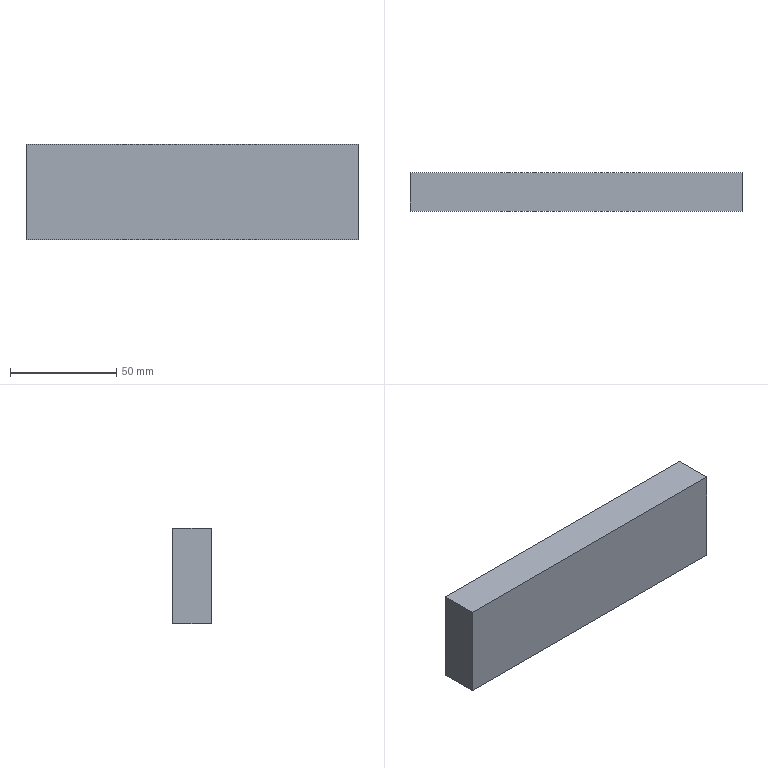NC program | NX | posted with a generic post | part box 156 x 18 x 45 mm
Lines 1295 to 2242 of 3545:
(PLANAR_PROFILING , TOOL : D8C)
N2540 T06 M6
N2542 G53
N2544 G17 G0 G90 X-157.794 Y11.317 S3500 M3
N2546 G43 Z19.87 H6
N2548 Z2.8
N2550 G94 G1 Z-0.2 F2000.
N2552 G3 X-152.934 Y11.934 R4.
N2554 G1 X-151.934 Y12.934
N2556 G2 X-149. Y14.15 R4.15
N2558 G1 X-27.15
N2560 Y39.
N2562 G2 X-25.934 Y41.934 R4.15
N2564 G1 X-24.934 Y42.934
N2566 G2 X-22. Y44.15 R4.15
N2568 G1 X-1.
N2570 G2 X1.934 Y42.934 R4.15
N2572 G1 X2.934 Y41.934
N2574 G3 X7.794 Y41.317 R4.
N2576 G1 Z2.8
N2578 G0 Z2.6
N2580 G1 Z-0.4
N2582 G2 X2.934 Y41.934 R4.
N2584 G1 X1.934 Y42.934
N2586 G3 X-1. Y44.15 R4.15
N2588 G1 X-22.
N2590 G3 X-24.934 Y42.934 R4.15
N2592 G1 X-25.934 Y41.934
N2594 G3 X-27.15 Y39. R4.15
N2596 G1 Y14.15
N2598 X-149.
N2600 G3 X-151.934 Y12.934 R4.15
N2602 G1 X-152.934 Y11.934
N2604 G2 X-157.794 Y11.317 R4.
N2606 G1 Z2.6
N2608 G0 Z2.4
N2610 G1 Z-0.6
N2612 G3 X-152.934 Y11.934 R4.
N2614 G1 X-151.934 Y12.934
N2616 G2 X-149. Y14.15 R4.15
N2618 G1 X-27.15
N2620 Y39.
N2622 G2 X-25.934 Y41.934 R4.15
N2624 G1 X-24.934 Y42.934
N2626 G2 X-22. Y44.15 R4.15
N2628 G1 X-1.
N2630 G2 X1.934 Y42.934 R4.15
N2632 G1 X2.934 Y41.934
N2634 G3 X7.794 Y41.317 R4.
N2636 G1 Z2.4
N2638 G0 Z2.2
N2640 G1 Z-0.8
N2642 G2 X2.934 Y41.934 R4.
N2644 G1 X1.934 Y42.934
N2646 G3 X-1. Y44.15 R4.15
N2648 G1 X-22.
N2650 G3 X-24.934 Y42.934 R4.15
N2652 G1 X-25.934 Y41.934
N2654 G3 X-27.15 Y39. R4.15
N2656 G1 Y14.15
N2658 X-149.
N2660 G3 X-151.934 Y12.934 R4.15
N2662 G1 X-152.934 Y11.934
N2664 G2 X-157.794 Y11.317 R4.
N2666 G1 Z2.2
N2668 G0 Z2.
N2670 G1 Z-1.
N2672 G3 X-152.934 Y11.934 R4.
N2674 G1 X-151.934 Y12.934
N2676 G2 X-149. Y14.15 R4.15
N2678 G1 X-27.15
N2680 Y39.
N2682 G2 X-25.934 Y41.934 R4.15
N2684 G1 X-24.934 Y42.934
N2686 G2 X-22. Y44.15 R4.15
N2688 G1 X-1.
N2690 G2 X1.934 Y42.934 R4.15
N2692 G1 X2.934 Y41.934
N2694 G3 X7.794 Y41.317 R4.
N2696 G1 Z2.
N2698 G0 Z1.8
N2700 G1 Z-1.2
N2702 G2 X2.934 Y41.934 R4.
N2704 G1 X1.934 Y42.934
N2706 G3 X-1. Y44.15 R4.15
N2708 G1 X-22.
N2710 G3 X-24.934 Y42.934 R4.15
N2712 G1 X-25.934 Y41.934
N2714 G3 X-27.15 Y39. R4.15
N2716 G1 Y14.15
N2718 X-149.
N2720 G3 X-151.934 Y12.934 R4.15
N2722 G1 X-152.934 Y11.934
N2724 G2 X-157.794 Y11.317 R4.
N2726 G1 Z1.8
N2728 G0 Z1.6
N2730 G1 Z-1.4
N2732 G3 X-152.934 Y11.934 R4.
N2734 G1 X-151.934 Y12.934
N2736 G2 X-149. Y14.15 R4.15
N2738 G1 X-27.15
N2740 Y39.
N2742 G2 X-25.934 Y41.934 R4.15
N2744 G1 X-24.934 Y42.934
N2746 G2 X-22. Y44.15 R4.15
N2748 G1 X-1.
N2750 G2 X1.934 Y42.934 R4.15
N2752 G1 X2.934 Y41.934
N2754 G3 X7.794 Y41.317 R4.
N2756 G1 Z1.6
N2758 G0 Z1.4
N2760 G1 Z-1.6
N2762 G2 X2.934 Y41.934 R4.
N2764 G1 X1.934 Y42.934
N2766 G3 X-1. Y44.15 R4.15
N2768 G1 X-22.
N2770 G3 X-24.934 Y42.934 R4.15
N2772 G1 X-25.934 Y41.934
N2774 G3 X-27.15 Y39. R4.15
N2776 G1 Y14.15
N2778 X-149.
N2780 G3 X-151.934 Y12.934 R4.15
N2782 G1 X-152.934 Y11.934
N2784 G2 X-157.794 Y11.317 R4.
N2786 G1 Z1.4
N2788 G0 Z1.2
N2790 G1 Z-1.8
N2792 G3 X-152.934 Y11.934 R4.
N2794 G1 X-151.934 Y12.934
N2796 G2 X-149. Y14.15 R4.15
N2798 G1 X-27.15
N2800 Y39.
N2802 G2 X-25.934 Y41.934 R4.15
N2804 G1 X-24.934 Y42.934
N2806 G2 X-22. Y44.15 R4.15
N2808 G1 X-1.
N2810 G2 X1.934 Y42.934 R4.15
N2812 G1 X2.934 Y41.934
N2814 G3 X7.794 Y41.317 R4.
N2816 G1 Z1.2
N2818 G0 Z1.
N2820 G1 Z-2.
N2822 G2 X2.934 Y41.934 R4.
N2824 G1 X1.934 Y42.934
N2826 G3 X-1. Y44.15 R4.15
N2828 G1 X-22.
N2830 G3 X-24.934 Y42.934 R4.15
N2832 G1 X-25.934 Y41.934
N2834 G3 X-27.15 Y39. R4.15
N2836 G1 Y14.15
N2838 X-149.
N2840 G3 X-151.934 Y12.934 R4.15
N2842 G1 X-152.934 Y11.934
N2844 G2 X-157.794 Y11.317 R4.
N2846 G1 Z1.
N2848 G0 Z0.8
N2850 G1 Z-2.2
N2852 G3 X-152.934 Y11.934 R4.
N2854 G1 X-151.934 Y12.934
N2856 G2 X-149. Y14.15 R4.15
N2858 G1 X-27.15
N2860 Y39.
N2862 G2 X-25.934 Y41.934 R4.15
N2864 G1 X-24.934 Y42.934
N2866 G2 X-22. Y44.15 R4.15
N2868 G1 X-1.
N2870 G2 X1.934 Y42.934 R4.15
N2872 G1 X2.934 Y41.934
N2874 G3 X7.794 Y41.317 R4.
N2876 G1 Z0.8
N2878 G0 Z0.6
N2880 G1 Z-2.4
N2882 G2 X2.934 Y41.934 R4.
N2884 G1 X1.934 Y42.934
N2886 G3 X-1. Y44.15 R4.15
N2888 G1 X-22.
N2890 G3 X-24.934 Y42.934 R4.15
N2892 G1 X-25.934 Y41.934
N2894 G3 X-27.15 Y39. R4.15
N2896 G1 Y14.15
N2898 X-149.
N2900 G3 X-151.934 Y12.934 R4.15
N2902 G1 X-152.934 Y11.934
N2904 G2 X-157.794 Y11.317 R4.
N2906 G1 Z0.6
N2908 G0 Z0.4
N2910 G1 Z-2.6
N2912 G3 X-152.934 Y11.934 R4.
N2914 G1 X-151.934 Y12.934
N2916 G2 X-149. Y14.15 R4.15
N2918 G1 X-27.15
N2920 Y39.
N2922 G2 X-25.934 Y41.934 R4.15
N2924 G1 X-24.934 Y42.934
N2926 G2 X-22. Y44.15 R4.15
N2928 G1 X-1.
N2930 G2 X1.934 Y42.934 R4.15
N2932 G1 X2.934 Y41.934
N2934 G3 X7.794 Y41.317 R4.
N2936 G1 Z0.4
N2938 G0 Z0.2
N2940 G1 Z-2.8
N2942 G2 X2.934 Y41.934 R4.
N2944 G1 X1.934 Y42.934
N2946 G3 X-1. Y44.15 R4.15
N2948 G1 X-22.
N2950 G3 X-24.934 Y42.934 R4.15
N2952 G1 X-25.934 Y41.934
N2954 G3 X-27.15 Y39. R4.15
N2956 G1 Y14.15
N2958 X-149.
N2960 G3 X-151.934 Y12.934 R4.15
N2962 G1 X-152.934 Y11.934
N2964 G2 X-157.794 Y11.317 R4.
N2966 G1 Z0.2
N2968 G0 Z0.
N2970 G1 Z-3.
N2972 G3 X-152.934 Y11.934 R4.
N2974 G1 X-151.934 Y12.934
N2976 G2 X-149. Y14.15 R4.15
N2978 G1 X-27.15
N2980 Y39.
N2982 G2 X-25.934 Y41.934 R4.15
N2984 G1 X-24.934 Y42.934
N2986 G2 X-22. Y44.15 R4.15
N2988 G1 X-1.
N2990 G2 X1.934 Y42.934 R4.15
N2992 G1 X2.934 Y41.934
N2994 G3 X7.794 Y41.317 R4.
N2996 G1 Z0.
N2998 G0 Z-0.2
N3000 G1 Z-3.2
N3002 G2 X2.934 Y41.934 R4.
N3004 G1 X1.934 Y42.934
N3006 G3 X-1. Y44.15 R4.15
N3008 G1 X-22.
N3010 G3 X-24.934 Y42.934 R4.15
N3012 G1 X-25.934 Y41.934
N3014 G3 X-27.15 Y39. R4.15
N3016 G1 Y14.15
N3018 X-149.
N3020 G3 X-151.934 Y12.934 R4.15
N3022 G1 X-152.934 Y11.934
N3024 G2 X-157.794 Y11.317 R4.
N3026 G1 Z-0.2
N3028 G0 Z-0.4
N3030 G1 Z-3.4
N3032 G3 X-152.934 Y11.934 R4.
N3034 G1 X-151.934 Y12.934
N3036 G2 X-149. Y14.15 R4.15
N3038 G1 X-27.15
N3040 Y39.
N3042 G2 X-25.934 Y41.934 R4.15
N3044 G1 X-24.934 Y42.934
N3046 G2 X-22. Y44.15 R4.15
N3048 G1 X-1.
N3050 G2 X1.934 Y42.934 R4.15
N3052 G1 X2.934 Y41.934
N3054 G3 X7.794 Y41.317 R4.
N3056 G1 Z-0.4
N3058 G0 Z-0.6
N3060 G1 Z-3.6
N3062 G2 X2.934 Y41.934 R4.
N3064 G1 X1.934 Y42.934
N3066 G3 X-1. Y44.15 R4.15
N3068 G1 X-22.
N3070 G3 X-24.934 Y42.934 R4.15
N3072 G1 X-25.934 Y41.934
N3074 G3 X-27.15 Y39. R4.15
N3076 G1 Y14.15
N3078 X-149.
N3080 G3 X-151.934 Y12.934 R4.15
N3082 G1 X-152.934 Y11.934
N3084 G2 X-157.794 Y11.317 R4.
N3086 G1 Z-0.6
N3088 G0 Z-0.8
N3090 G1 Z-3.8
N3092 G3 X-152.934 Y11.934 R4.
N3094 G1 X-151.934 Y12.934
N3096 G2 X-149. Y14.15 R4.15
N3098 G1 X-27.15
N3100 Y39.
N3102 G2 X-25.934 Y41.934 R4.15
N3104 G1 X-24.934 Y42.934
N3106 G2 X-22. Y44.15 R4.15
N3108 G1 X-1.
N3110 G2 X1.934 Y42.934 R4.15
N3112 G1 X2.934 Y41.934
N3114 G3 X7.794 Y41.317 R4.
N3116 G1 Z-0.8
N3118 G0 Z-1.
N3120 G1 Z-4.
N3122 G2 X2.934 Y41.934 R4.
N3124 G1 X1.934 Y42.934
N3126 G3 X-1. Y44.15 R4.15
N3128 G1 X-22.
N3130 G3 X-24.934 Y42.934 R4.15
N3132 G1 X-25.934 Y41.934
N3134 G3 X-27.15 Y39. R4.15
N3136 G1 Y14.15
N3138 X-149.
N3140 G3 X-151.934 Y12.934 R4.15
N3142 G1 X-152.934 Y11.934
N3144 G2 X-157.794 Y11.317 R4.
N3146 G1 Z-1.
N3148 G0 Z-1.2
N3150 G1 Z-4.2
N3152 G3 X-152.934 Y11.934 R4.
N3154 G1 X-151.934 Y12.934
N3156 G2 X-149. Y14.15 R4.15
N3158 G1 X-27.15
N3160 Y39.
N3162 G2 X-25.934 Y41.934 R4.15
N3164 G1 X-24.934 Y42.934
N3166 G2 X-22. Y44.15 R4.15
N3168 G1 X-1.
N3170 G2 X1.934 Y42.934 R4.15
N3172 G1 X2.934 Y41.934
N3174 G3 X7.794 Y41.317 R4.
N3176 G1 Z-1.2
N3178 G0 Z-1.4
N3180 G1 Z-4.4
N3182 G2 X2.934 Y41.934 R4.
N3184 G1 X1.934 Y42.934
N3186 G3 X-1. Y44.15 R4.15
N3188 G1 X-22.
N3190 G3 X-24.934 Y42.934 R4.15
N3192 G1 X-25.934 Y41.934
N3194 G3 X-27.15 Y39. R4.15
N3196 G1 Y14.15
N3198 X-149.
N3200 G3 X-151.934 Y12.934 R4.15
N3202 G1 X-152.934 Y11.934
N3204 G2 X-157.794 Y11.317 R4.
N3206 G1 Z-1.4
N3208 G0 Z-1.6
N3210 G1 Z-4.6
N3212 G3 X-152.934 Y11.934 R4.
N3214 G1 X-151.934 Y12.934
N3216 G2 X-149. Y14.15 R4.15
N3218 G1 X-27.15
N3220 Y39.
N3222 G2 X-25.934 Y41.934 R4.15
N3224 G1 X-24.934 Y42.934
N3226 G2 X-22. Y44.15 R4.15
N3228 G1 X-1.
N3230 G2 X1.934 Y42.934 R4.15
N3232 G1 X2.934 Y41.934
N3234 G3 X7.794 Y41.317 R4.
N3236 G1 Z-1.6
N3238 G0 Z-1.8
N3240 G1 Z-4.8
N3242 G2 X2.934 Y41.934 R4.
N3244 G1 X1.934 Y42.934
N3246 G3 X-1. Y44.15 R4.15
N3248 G1 X-22.
N3250 G3 X-24.934 Y42.934 R4.15
N3252 G1 X-25.934 Y41.934
N3254 G3 X-27.15 Y39. R4.15
N3256 G1 Y14.15
N3258 X-149.
N3260 G3 X-151.934 Y12.934 R4.15
N3262 G1 X-152.934 Y11.934
N3264 G2 X-157.794 Y11.317 R4.
N3266 G1 Z-1.8
N3268 G0 Z-2.
N3270 G1 Z-5.
N3272 G3 X-152.934 Y11.934 R4.
N3274 G1 X-151.934 Y12.934
N3276 G2 X-149. Y14.15 R4.15
N3278 G1 X-27.15
N3280 Y39.
N3282 G2 X-25.934 Y41.934 R4.15
N3284 G1 X-24.934 Y42.934
N3286 G2 X-22. Y44.15 R4.15
N3288 G1 X-1.
N3290 G2 X1.934 Y42.934 R4.15
N3292 G1 X2.934 Y41.934
N3294 G3 X7.794 Y41.317 R4.
N3296 G1 Z-2.
N3298 G0 Z-2.2
N3300 G1 Z-5.2
N3302 G2 X2.934 Y41.934 R4.
N3304 G1 X1.934 Y42.934
N3306 G3 X-1. Y44.15 R4.15
N3308 G1 X-22.
N3310 G3 X-24.934 Y42.934 R4.15
N3312 G1 X-25.934 Y41.934
N3314 G3 X-27.15 Y39. R4.15
N3316 G1 Y14.15
N3318 X-149.
N3320 G3 X-151.934 Y12.934 R4.15
N3322 G1 X-152.934 Y11.934
N3324 G2 X-157.794 Y11.317 R4.
N3326 G1 Z-2.2
N3328 G0 Z-2.4
N3330 G1 Z-5.4
N3332 G3 X-152.934 Y11.934 R4.
N3334 G1 X-151.934 Y12.934
N3336 G2 X-149. Y14.15 R4.15
N3338 G1 X-27.15
N3340 Y39.
N3342 G2 X-25.934 Y41.934 R4.15
N3344 G1 X-24.934 Y42.934
N3346 G2 X-22. Y44.15 R4.15
N3348 G1 X-1.
N3350 G2 X1.934 Y42.934 R4.15
N3352 G1 X2.934 Y41.934
N3354 G3 X7.794 Y41.317 R4.
N3356 G1 Z-2.4
N3358 G0 Z-2.6
N3360 G1 Z-5.6
N3362 G2 X2.934 Y41.934 R4.
N3364 G1 X1.934 Y42.934
N3366 G3 X-1. Y44.15 R4.15
N3368 G1 X-22.
N3370 G3 X-24.934 Y42.934 R4.15
N3372 G1 X-25.934 Y41.934
N3374 G3 X-27.15 Y39. R4.15
N3376 G1 Y14.15
N3378 X-149.
N3380 G3 X-151.934 Y12.934 R4.15
N3382 G1 X-152.934 Y11.934
N3384 G2 X-157.794 Y11.317 R4.
N3386 G1 Z-2.6
N3388 G0 Z-2.8
N3390 G1 Z-5.8
N3392 G3 X-152.934 Y11.934 R4.
N3394 G1 X-151.934 Y12.934
N3396 G2 X-149. Y14.15 R4.15
N3398 G1 X-27.15
N3400 Y39.
N3402 G2 X-25.934 Y41.934 R4.15
N3404 G1 X-24.934 Y42.934
N3406 G2 X-22. Y44.15 R4.15
N3408 G1 X-1.
N3410 G2 X1.934 Y42.934 R4.15
N3412 G1 X2.934 Y41.934
N3414 G3 X7.794 Y41.317 R4.
N3416 G1 Z-2.8
N3418 G0 Z-3.
N3420 G1 Z-6.
N3422 G2 X2.934 Y41.934 R4.
N3424 G1 X1.934 Y42.934
N3426 G3 X-1. Y44.15 R4.15
N3428 G1 X-22.
N3430 G3 X-24.934 Y42.934 R4.15
N3432 G1 X-25.934 Y41.934
N3434 G3 X-27.15 Y39. R4.15
N3436 G1 Y14.15
N3438 X-149.
N3440 G3 X-151.934 Y12.934 R4.15
N3442 G1 X-152.934 Y11.934
N3444 G2 X-157.794 Y11.317 R4.
N3446 G1 Z-3.
N3448 G0 Z-3.2
N3450 G1 Z-6.2
N3452 G3 X-152.934 Y11.934 R4.
N3454 G1 X-151.934 Y12.934
N3456 G2 X-149. Y14.15 R4.15
N3458 G1 X-27.15
N3460 Y39.
N3462 G2 X-25.934 Y41.934 R4.15
N3464 G1 X-24.934 Y42.934
N3466 G2 X-22. Y44.15 R4.15
N3468 G1 X-1.
N3470 G2 X1.934 Y42.934 R4.15
N3472 G1 X2.934 Y41.934
N3474 G3 X7.794 Y41.317 R4.
N3476 G1 Z-3.2
N3478 G0 Z-3.4
N3480 G1 Z-6.4
N3482 G2 X2.934 Y41.934 R4.
N3484 G1 X1.934 Y42.934
N3486 G3 X-1. Y44.15 R4.15
N3488 G1 X-22.
N3490 G3 X-24.934 Y42.934 R4.15
N3492 G1 X-25.934 Y41.934
N3494 G3 X-27.15 Y39. R4.15
N3496 G1 Y14.15
N3498 X-149.
N3500 G3 X-151.934 Y12.934 R4.15
N3502 G1 X-152.934 Y11.934
N3504 G2 X-157.794 Y11.317 R4.
N3506 G1 Z-3.4
N3508 G0 Z-3.6
N3510 G1 Z-6.6
N3512 G3 X-152.934 Y11.934 R4.
N3514 G1 X-151.934 Y12.934
N3516 G2 X-149. Y14.15 R4.15
N3518 G1 X-27.15
N3520 Y39.
N3522 G2 X-25.934 Y41.934 R4.15
N3524 G1 X-24.934 Y42.934
N3526 G2 X-22. Y44.15 R4.15
N3528 G1 X-1.
N3530 G2 X1.934 Y42.934 R4.15
N3532 G1 X2.934 Y41.934
N3534 G3 X7.794 Y41.317 R4.
N3536 G1 Z-3.6
N3538 G0 Z-3.8
N3540 G1 Z-6.8
N3542 G2 X2.934 Y41.934 R4.
N3544 G1 X1.934 Y42.934
N3546 G3 X-1. Y44.15 R4.15
N3548 G1 X-22.
N3550 G3 X-24.934 Y42.934 R4.15
N3552 G1 X-25.934 Y41.934
N3554 G3 X-27.15 Y39. R4.15
N3556 G1 Y14.15
N3558 X-149.
N3560 G3 X-151.934 Y12.934 R4.15
N3562 G1 X-152.934 Y11.934
N3564 G2 X-157.794 Y11.317 R4.
N3566 G1 Z-3.8
N3568 G0 Z-4.
N3570 G1 Z-7.
N3572 G3 X-152.934 Y11.934 R4.
N3574 G1 X-151.934 Y12.934
N3576 G2 X-149. Y14.15 R4.15
N3578 G1 X-27.15
N3580 Y39.
N3582 G2 X-25.934 Y41.934 R4.15
N3584 G1 X-24.934 Y42.934
N3586 G2 X-22. Y44.15 R4.15
N3588 G1 X-1.
N3590 G2 X1.934 Y42.934 R4.15
N3592 G1 X2.934 Y41.934
N3594 G3 X7.794 Y41.317 R4.
N3596 G1 Z-4.
N3598 G0 Z-4.2
N3600 G1 Z-7.2
N3602 G2 X2.934 Y41.934 R4.
N3604 G1 X1.934 Y42.934
N3606 G3 X-1. Y44.15 R4.15
N3608 G1 X-22.
N3610 G3 X-24.934 Y42.934 R4.15
N3612 G1 X-25.934 Y41.934
N3614 G3 X-27.15 Y39. R4.15
N3616 G1 Y14.15
N3618 X-149.
N3620 G3 X-151.934 Y12.934 R4.15
N3622 G1 X-152.934 Y11.934
N3624 G2 X-157.794 Y11.317 R4.
N3626 G1 Z-4.2
N3628 G0 Z-4.4
N3630 G1 Z-7.4
N3632 G3 X-152.934 Y11.934 R4.
N3634 G1 X-151.934 Y12.934
N3636 G2 X-149. Y14.15 R4.15
N3638 G1 X-27.15
N3640 Y39.
N3642 G2 X-25.934 Y41.934 R4.15
N3644 G1 X-24.934 Y42.934
N3646 G2 X-22. Y44.15 R4.15
N3648 G1 X-1.
N3650 G2 X1.934 Y42.934 R4.15
N3652 G1 X2.934 Y41.934
N3654 G3 X7.794 Y41.317 R4.
N3656 G1 Z-4.4
N3658 G0 Z-4.6
N3660 G1 Z-7.6
N3662 G2 X2.934 Y41.934 R4.
N3664 G1 X1.934 Y42.934
N3666 G3 X-1. Y44.15 R4.15
N3668 G1 X-22.
N3670 G3 X-24.934 Y42.934 R4.15
N3672 G1 X-25.934 Y41.934
N3674 G3 X-27.15 Y39. R4.15
N3676 G1 Y14.15
N3678 X-149.
N3680 G3 X-151.934 Y12.934 R4.15
N3682 G1 X-152.934 Y11.934
N3684 G2 X-157.794 Y11.317 R4.
N3686 G1 Z-4.6
N3688 G0 Z-4.8
N3690 G1 Z-7.8
N3692 G3 X-152.934 Y11.934 R4.
N3694 G1 X-151.934 Y12.934
N3696 G2 X-149. Y14.15 R4.15
N3698 G1 X-27.15
N3700 Y39.
N3702 G2 X-25.934 Y41.934 R4.15
N3704 G1 X-24.934 Y42.934
N3706 G2 X-22. Y44.15 R4.15
N3708 G1 X-1.
N3710 G2 X1.934 Y42.934 R4.15
N3712 G1 X2.934 Y41.934
N3714 G3 X7.794 Y41.317 R4.
N3716 G1 Z-4.8
N3718 G0 Z-5.
N3720 G1 Z-8.
N3722 G2 X2.934 Y41.934 R4.
N3724 G1 X1.934 Y42.934
N3726 G3 X-1. Y44.15 R4.15
N3728 G1 X-22.
N3730 G3 X-24.934 Y42.934 R4.15
N3732 G1 X-25.934 Y41.934
N3734 G3 X-27.15 Y39. R4.15
N3736 G1 Y14.15
N3738 X-149.
N3740 G3 X-151.934 Y12.934 R4.15
N3742 G1 X-152.934 Y11.934
N3744 G2 X-157.794 Y11.317 R4.
N3746 G1 Z-5.
N3748 G0 Z-5.2
N3750 G1 Z-8.2
N3752 G3 X-152.934 Y11.934 R4.
N3754 G1 X-151.934 Y12.934
N3756 G2 X-149. Y14.15 R4.15
N3758 G1 X-27.15
N3760 Y39.
N3762 G2 X-25.934 Y41.934 R4.15
N3764 G1 X-24.934 Y42.934
N3766 G2 X-22. Y44.15 R4.15
N3768 G1 X-1.
N3770 G2 X1.934 Y42.934 R4.15
N3772 G1 X2.934 Y41.934
N3774 G3 X7.794 Y41.317 R4.
N3776 G1 Z-5.2
N3778 G0 Z-5.4
N3780 G1 Z-8.4
N3782 G2 X2.934 Y41.934 R4.
N3784 G1 X1.934 Y42.934
N3786 G3 X-1. Y44.15 R4.15
N3788 G1 X-22.
N3790 G3 X-24.934 Y42.934 R4.15
N3792 G1 X-25.934 Y41.934
N3794 G3 X-27.15 Y39. R4.15
N3796 G1 Y14.15
N3798 X-149.
N3800 G3 X-151.934 Y12.934 R4.15
N3802 G1 X-152.934 Y11.934
N3804 G2 X-157.794 Y11.317 R4.
N3806 G1 Z-5.4
N3808 G0 Z-5.6
N3810 G1 Z-8.6
N3812 G3 X-152.934 Y11.934 R4.
N3814 G1 X-151.934 Y12.934
N3816 G2 X-149. Y14.15 R4.15
N3818 G1 X-27.15
N3820 Y39.
N3822 G2 X-25.934 Y41.934 R4.15
N3824 G1 X-24.934 Y42.934
N3826 G2 X-22. Y44.15 R4.15
N3828 G1 X-1.
N3830 G2 X1.934 Y42.934 R4.15
N3832 G1 X2.934 Y41.934
N3834 G3 X7.794 Y41.317 R4.
N3836 G1 Z-5.6
N3838 G0 Z-5.8
N3840 G1 Z-8.8
N3842 G2 X2.934 Y41.934 R4.
N3844 G1 X1.934 Y42.934
N3846 G3 X-1. Y44.15 R4.15
N3848 G1 X-22.
N3850 G3 X-24.934 Y42.934 R4.15
N3852 G1 X-25.934 Y41.934
N3854 G3 X-27.15 Y39. R4.15
N3856 G1 Y14.15
N3858 X-149.
N3860 G3 X-151.934 Y12.934 R4.15
N3862 G1 X-152.934 Y11.934
N3864 G2 X-157.794 Y11.317 R4.
N3866 G1 Z-5.8
N3868 G0 Z-6.
N3870 G1 Z-9.
N3872 G3 X-152.934 Y11.934 R4.
N3874 G1 X-151.934 Y12.934
N3876 G2 X-149. Y14.15 R4.15
N3878 G1 X-27.15
N3880 Y39.
N3882 G2 X-25.934 Y41.934 R4.15
N3884 G1 X-24.934 Y42.934
N3886 G2 X-22. Y44.15 R4.15
N3888 G1 X-1.
N3890 G2 X1.934 Y42.934 R4.15
N3892 G1 X2.934 Y41.934
N3894 G3 X7.794 Y41.317 R4.
N3896 G1 Z-6.
N3898 G0 Z-6.2
N3900 G1 Z-9.2
N3902 G2 X2.934 Y41.934 R4.
N3904 G1 X1.934 Y42.934
N3906 G3 X-1. Y44.15 R4.15
N3908 G1 X-22.
N3910 G3 X-24.934 Y42.934 R4.15
N3912 G1 X-25.934 Y41.934
N3914 G3 X-27.15 Y39. R4.15
N3916 G1 Y14.15
N3918 X-149.
N3920 G3 X-151.934 Y12.934 R4.15
N3922 G1 X-152.934 Y11.934
N3924 G2 X-157.794 Y11.317 R4.
N3926 G1 Z-6.2
N3928 G0 Z-6.4
N3930 G1 Z-9.4
N3932 G3 X-152.934 Y11.934 R4.
N3934 G1 X-151.934 Y12.934
N3936 G2 X-149. Y14.15 R4.15
N3938 G1 X-27.15
N3940 Y39.
N3942 G2 X-25.934 Y41.934 R4.15
N3944 G1 X-24.934 Y42.934
N3946 G2 X-22. Y44.15 R4.15
N3948 G1 X-1.
N3950 G2 X1.934 Y42.934 R4.15
N3952 G1 X2.934 Y41.934
N3954 G3 X7.794 Y41.317 R4.
N3956 G1 Z-6.4
N3958 G0 Z-6.6
N3960 G1 Z-9.6
N3962 G2 X2.934 Y41.934 R4.
N3964 G1 X1.934 Y42.934
N3966 G3 X-1. Y44.15 R4.15
N3968 G1 X-22.
N3970 G3 X-24.934 Y42.934 R4.15
N3972 G1 X-25.934 Y41.934
N3974 G3 X-27.15 Y39. R4.15
N3976 G1 Y14.15
N3978 X-149.
N3980 G3 X-151.934 Y12.934 R4.15
N3982 G1 X-152.934 Y11.934
N3984 G2 X-157.794 Y11.317 R4.
N3986 G1 Z-6.6
N3988 G0 Z-6.8
N3990 G1 Z-9.8
N3992 G3 X-152.934 Y11.934 R4.
N3994 G1 X-151.934 Y12.934
N3996 G2 X-149. Y14.15 R4.15
N3998 G1 X-27.15
N4000 Y39.
N4002 G2 X-25.934 Y41.934 R4.15
N4004 G1 X-24.934 Y42.934
N4006 G2 X-22. Y44.15 R4.15
N4008 G1 X-1.
N4010 G2 X1.934 Y42.934 R4.15
N4012 G1 X2.934 Y41.934
N4014 G3 X7.794 Y41.317 R4.
N4016 G1 Z-6.8
N4018 G0 Z-7.
N4020 G1 Z-10.
N4022 G2 X2.934 Y41.934 R4.
N4024 G1 X1.934 Y42.934
N4026 G3 X-1. Y44.15 R4.15
N4028 G1 X-22.
N4030 G3 X-24.934 Y42.934 R4.15
N4032 G1 X-25.934 Y41.934
N4034 G3 X-27.15 Y39. R4.15
N4036 G1 Y14.15
N4038 X-149.
N4040 G3 X-151.934 Y12.934 R4.15
N4042 G1 X-152.934 Y11.934
N4044 G2 X-157.794 Y11.317 R4.
N4046 G1 Z-7.
N4048 G0 Z-7.2
N4050 G1 Z-10.2
N4052 G3 X-152.934 Y11.934 R4.
N4054 G1 X-151.934 Y12.934
N4056 G2 X-149. Y14.15 R4.15
N4058 G1 X-27.15
N4060 Y39.
N4062 G2 X-25.934 Y41.934 R4.15
N4064 G1 X-24.934 Y42.934
N4066 G2 X-22. Y44.15 R4.15
N4068 G1 X-1.
N4070 G2 X1.934 Y42.934 R4.15
N4072 G1 X2.934 Y41.934
N4074 G3 X7.794 Y41.317 R4.
N4076 G1 Z-7.2
N4078 G0 Z-7.4
N4080 G1 Z-10.4
N4082 G2 X2.934 Y41.934 R4.
N4084 G1 X1.934 Y42.934
N4086 G3 X-1. Y44.15 R4.15
N4088 G1 X-22.
N4090 G3 X-24.934 Y42.934 R4.15
N4092 G1 X-25.934 Y41.934
N4094 G3 X-27.15 Y39. R4.15
N4096 G1 Y14.15
N4098 X-149.
N4100 G3 X-151.934 Y12.934 R4.15
N4102 G1 X-152.934 Y11.934
N4104 G2 X-157.794 Y11.317 R4.
N4106 G1 Z-7.4
N4108 G0 Z-7.6
N4110 G1 Z-10.6
N4112 G3 X-152.934 Y11.934 R4.
N4114 G1 X-151.934 Y12.934
N4116 G2 X-149. Y14.15 R4.15
N4118 G1 X-27.15
N4120 Y39.
N4122 G2 X-25.934 Y41.934 R4.15
N4124 G1 X-24.934 Y42.934
N4126 G2 X-22. Y44.15 R4.15
N4128 G1 X-1.
N4130 G2 X1.934 Y42.934 R4.15
N4132 G1 X2.934 Y41.934
N4134 G3 X7.794 Y41.317 R4.
N4136 G1 Z-7.6
N4138 G0 Z-7.8
N4140 G1 Z-10.8
N4142 G2 X2.934 Y41.934 R4.
N4144 G1 X1.934 Y42.934
N4146 G3 X-1. Y44.15 R4.15
N4148 G1 X-22.
N4150 G3 X-24.934 Y42.934 R4.15
N4152 G1 X-25.934 Y41.934
N4154 G3 X-27.15 Y39. R4.15
N4156 G1 Y14.15
N4158 X-149.
N4160 G3 X-151.934 Y12.934 R4.15
N4162 G1 X-152.934 Y11.934
N4164 G2 X-157.794 Y11.317 R4.
N4166 G1 Z-7.8
N4168 G0 Z-8.
N4170 G1 Z-11.
N4172 G3 X-152.934 Y11.934 R4.
N4174 G1 X-151.934 Y12.934
N4176 G2 X-149. Y14.15 R4.15
N4178 G1 X-27.15
N4180 Y39.
N4182 G2 X-25.934 Y41.934 R4.15
N4184 G1 X-24.934 Y42.934
N4186 G2 X-22. Y44.15 R4.15
N4188 G1 X-1.
N4190 G2 X1.934 Y42.934 R4.15
N4192 G1 X2.934 Y41.934
N4194 G3 X7.794 Y41.317 R4.
N4196 G1 Z-8.
N4198 G0 Z-8.2
N4200 G1 Z-11.2
N4202 G2 X2.934 Y41.934 R4.
N4204 G1 X1.934 Y42.934
N4206 G3 X-1. Y44.15 R4.15
N4208 G1 X-22.
N4210 G3 X-24.934 Y42.934 R4.15
N4212 G1 X-25.934 Y41.934
N4214 G3 X-27.15 Y39. R4.15
N4216 G1 Y14.15
N4218 X-149.
N4220 G3 X-151.934 Y12.934 R4.15
N4222 G1 X-152.934 Y11.934
N4224 G2 X-157.794 Y11.317 R4.
N4226 G1 Z-8.2
N4228 G0 Z-8.4
N4230 G1 Z-11.4
N4232 G3 X-152.934 Y11.934 R4.
N4234 G1 X-151.934 Y12.934
N4236 G2 X-149. Y14.15 R4.15
N4238 G1 X-27.15
N4240 Y39.
N4242 G2 X-25.934 Y41.934 R4.15
N4244 G1 X-24.934 Y42.934
N4246 G2 X-22. Y44.15 R4.15
N4248 G1 X-1.
N4250 G2 X1.934 Y42.934 R4.15
N4252 G1 X2.934 Y41.934
N4254 G3 X7.794 Y41.317 R4.
N4256 G1 Z-8.4
N4258 G0 Z-8.6
N4260 G1 Z-11.6
N4262 G2 X2.934 Y41.934 R4.
N4264 G1 X1.934 Y42.934
N4266 G3 X-1. Y44.15 R4.15
N4268 G1 X-22.
N4270 G3 X-24.934 Y42.934 R4.15
N4272 G1 X-25.934 Y41.934
N4274 G3 X-27.15 Y39. R4.15
N4276 G1 Y14.15
N4278 X-149.
N4280 G3 X-151.934 Y12.934 R4.15
N4282 G1 X-152.934 Y11.934
N4284 G2 X-157.794 Y11.317 R4.
N4286 G1 Z-8.6
N4288 G0 Z-8.8
N4290 G1 Z-11.8
N4292 G3 X-152.934 Y11.934 R4.
N4294 G1 X-151.934 Y12.934
N4296 G2 X-149. Y14.15 R4.15
N4298 G1 X-27.15
N4300 Y39.
N4302 G2 X-25.934 Y41.934 R4.15
N4304 G1 X-24.934 Y42.934
N4306 G2 X-22. Y44.15 R4.15
N4308 G1 X-1.
N4310 G2 X1.934 Y42.934 R4.15
N4312 G1 X2.934 Y41.934
N4314 G3 X7.794 Y41.317 R4.
N4316 G1 Z-8.8
N4318 G0 Z-9.
N4320 G1 Z-12.
N4322 G2 X2.934 Y41.934 R4.
N4324 G1 X1.934 Y42.934
N4326 G3 X-1. Y44.15 R4.15
N4328 G1 X-22.
N4330 G3 X-24.934 Y42.934 R4.15
N4332 G1 X-25.934 Y41.934
N4334 G3 X-27.15 Y39. R4.15
N4336 G1 Y14.15
N4338 X-149.
N4340 G3 X-151.934 Y12.934 R4.15
N4342 G1 X-152.934 Y11.934
N4344 G2 X-157.794 Y11.317 R4.
N4346 G1 Z-9.
N4348 G0 Z-9.2
N4350 G1 Z-12.2
N4352 G3 X-152.934 Y11.934 R4.
N4354 G1 X-151.934 Y12.934
N4356 G2 X-149. Y14.15 R4.15
N4358 G1 X-27.15
N4360 Y39.
N4362 G2 X-25.934 Y41.934 R4.15
N4364 G1 X-24.934 Y42.934
N4366 G2 X-22. Y44.15 R4.15
N4368 G1 X-1.
N4370 G2 X1.934 Y42.934 R4.15
N4372 G1 X2.934 Y41.934
N4374 G3 X7.794 Y41.317 R4.
N4376 G1 Z-9.2
N4378 G0 Z19.87
N4380 M5
(PLANAR_PROFILING_COPY , TOOL : D6J)
N4382 T07 M6
N4384 G53
N4386 G17 G0 G90 X-156.364 Y11.121 S3000 M3
N4388 G43 Z19.87 H7
N4390 Z-9.1
N4392 G94 G1 Z-12.1 F400.
N4394 G3 X-152.121 Y11.121 R3.
N4396 G1 X-151.121 Y12.121
N4398 G2 X-149. Y13. R3.
N4400 G1 X-26.
N4402 Y39.
N4404 G2 X-25.121 Y41.121 R3.
N4406 G1 X-24.121 Y42.121
N4408 G2 X-22. Y43. R3.
N4410 G1 X-1.
N4412 G2 X1.121 Y42.121 R3.
N4414 G1 X2.121 Y41.121
N4416 G3 X6.364 Y41.121 R3.
N4418 G1 Z-9.1
N4420 G0 Z19.87
N4422 M5